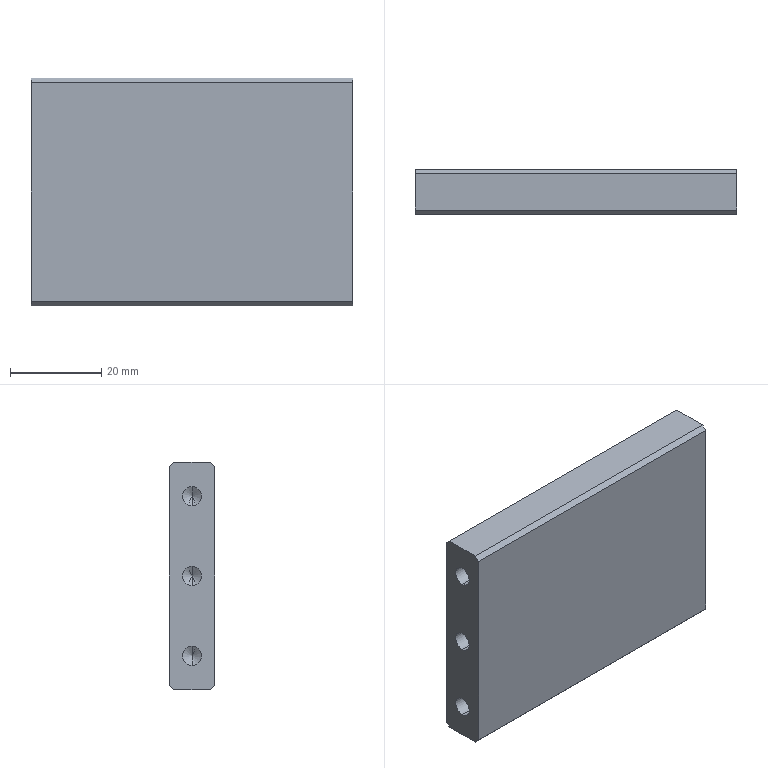Part | STEP file | 10000020443swp000-1 | 1 solid | 34 faces | box 70.5 x 10 x 50 mm | volume 33628 mm3 | cylinder 12 | cone 12 | plane 10 | commonest cylinder face diameters 4.2 x12
STEP:
#1=CARTESIAN_POINT('',(-17.85,5.,15.4));
#2=VERTEX_POINT('',#1);
#3=CARTESIAN_POINT('',(-17.85,5.,19.6));
#4=VERTEX_POINT('',#3);
#5=CARTESIAN_POINT('',(-17.85,5.,17.5));
#6=DIRECTION('',(-1.,0.,0.));
#7=DIRECTION('',(0.,0.,1.));
#8=AXIS2_PLACEMENT_3D('',#5,#6,#7);
#9=CIRCLE('',#8,2.1);
#10=EDGE_CURVE('',#2,#4,#9,.T.);
#11=ORIENTED_EDGE('',*,*,#10,.F.);
#12=CARTESIAN_POINT('',(-35.25,5.,15.4));
#13=VERTEX_POINT('',#12);
#14=CARTESIAN_POINT('',(-35.25,5.,15.4));
#15=DIRECTION('',(-1.,0.,0.));
#16=VECTOR('',#15,1000.);
#17=LINE('',#14,#16);
#18=EDGE_CURVE('',#2,#13,#17,.T.);
#19=ORIENTED_EDGE('',*,*,#18,.T.);
#20=CARTESIAN_POINT('',(-35.25,5.,19.6));
#21=VERTEX_POINT('',#20);
#22=CARTESIAN_POINT('',(-35.25,5.,17.5));
#23=DIRECTION('',(-1.,0.,0.));
#24=DIRECTION('',(0.,0.,1.));
#25=AXIS2_PLACEMENT_3D('',#22,#23,#24);
#26=CIRCLE('',#25,2.1);
#27=EDGE_CURVE('',#13,#21,#26,.T.);
#28=ORIENTED_EDGE('',*,*,#27,.T.);
#29=CARTESIAN_POINT('',(-35.25,5.,19.6));
#30=DIRECTION('',(-1.,0.,0.));
#31=VECTOR('',#30,1000.);
#32=LINE('',#29,#31);
#33=EDGE_CURVE('',#4,#21,#32,.T.);
#34=ORIENTED_EDGE('',*,*,#33,.F.);
#35=EDGE_LOOP('',(#11,#19,#28,#34));
#36=FACE_OUTER_BOUND('',#35,.T.);
#37=CARTESIAN_POINT('',(-35.25,5.,17.5));
#38=DIRECTION('',(-1.,0.,0.));
#39=DIRECTION('',(0.,0.,1.));
#40=AXIS2_PLACEMENT_3D('',#37,#38,#39);
#41=CYLINDRICAL_SURFACE('',#40,2.1);
#42=ADVANCED_FACE('',(#36),#41,.F.);
#43=CARTESIAN_POINT('',(-16.588,5.,17.5));
#44=VERTEX_POINT('',#43);
#45=CARTESIAN_POINT('',(-17.85,5.,19.6));
#46=DIRECTION('',(-0.515,0.,0.8572));
#47=VECTOR('',#46,1000.);
#48=LINE('',#45,#47);
#49=EDGE_CURVE('',#44,#4,#48,.T.);
#50=ORIENTED_EDGE('',*,*,#49,.F.);
#51=CARTESIAN_POINT('',(-17.85,5.,15.4));
#52=DIRECTION('',(-0.515,0.,-0.8572));
#53=VECTOR('',#52,1000.);
#54=LINE('',#51,#53);
#55=EDGE_CURVE('',#44,#2,#54,.T.);
#56=ORIENTED_EDGE('',*,*,#55,.T.);
#57=ORIENTED_EDGE('',*,*,#10,.T.);
#58=EDGE_LOOP('',(#50,#56,#57));
#59=FACE_OUTER_BOUND('',#58,.T.);
#60=CARTESIAN_POINT('',(-17.85,5.,17.5));
#61=DIRECTION('',(-1.,0.,0.));
#62=DIRECTION('',(0.,0.,1.));
#63=AXIS2_PLACEMENT_3D('',#60,#61,#62);
#64=CONICAL_SURFACE('',#63,2.1,1.03);
#65=ADVANCED_FACE('',(#59),#64,.F.);
#66=CARTESIAN_POINT('',(-17.85,5.,-2.1));
#67=VERTEX_POINT('',#66);
#68=CARTESIAN_POINT('',(-17.85,5.,2.1));
#69=VERTEX_POINT('',#68);
#70=CARTESIAN_POINT('',(-17.85,5.,0.));
#71=DIRECTION('',(-1.,0.,0.));
#72=DIRECTION('',(0.,0.,1.));
#73=AXIS2_PLACEMENT_3D('',#70,#71,#72);
#74=CIRCLE('',#73,2.1);
#75=EDGE_CURVE('',#67,#69,#74,.T.);
#76=ORIENTED_EDGE('',*,*,#75,.F.);
#77=CARTESIAN_POINT('',(-35.25,5.,-2.1));
#78=VERTEX_POINT('',#77);
#79=CARTESIAN_POINT('',(-35.25,5.,-2.1));
#80=DIRECTION('',(-1.,0.,0.));
#81=VECTOR('',#80,1000.);
#82=LINE('',#79,#81);
#83=EDGE_CURVE('',#67,#78,#82,.T.);
#84=ORIENTED_EDGE('',*,*,#83,.T.);
#85=CARTESIAN_POINT('',(-35.25,5.,2.1));
#86=VERTEX_POINT('',#85);
#87=CARTESIAN_POINT('',(-35.25,5.,0.));
#88=DIRECTION('',(-1.,0.,0.));
#89=DIRECTION('',(0.,0.,1.));
#90=AXIS2_PLACEMENT_3D('',#87,#88,#89);
#91=CIRCLE('',#90,2.1);
#92=EDGE_CURVE('',#78,#86,#91,.T.);
#93=ORIENTED_EDGE('',*,*,#92,.T.);
#94=CARTESIAN_POINT('',(-35.25,5.,2.1));
#95=DIRECTION('',(-1.,0.,0.));
#96=VECTOR('',#95,1000.);
#97=LINE('',#94,#96);
#98=EDGE_CURVE('',#69,#86,#97,.T.);
#99=ORIENTED_EDGE('',*,*,#98,.F.);
#100=EDGE_LOOP('',(#76,#84,#93,#99));
#101=FACE_OUTER_BOUND('',#100,.T.);
#102=CARTESIAN_POINT('',(-35.25,5.,0.));
#103=DIRECTION('',(-1.,0.,0.));
#104=DIRECTION('',(0.,0.,1.));
#105=AXIS2_PLACEMENT_3D('',#102,#103,#104);
#106=CYLINDRICAL_SURFACE('',#105,2.1);
#107=ADVANCED_FACE('',(#101),#106,.F.);
#108=CARTESIAN_POINT('',(-16.588,5.,0.));
#109=VERTEX_POINT('',#108);
#110=CARTESIAN_POINT('',(-17.85,5.,2.1));
#111=DIRECTION('',(-0.515,0.,0.8572));
#112=VECTOR('',#111,1000.);
#113=LINE('',#110,#112);
#114=EDGE_CURVE('',#109,#69,#113,.T.);
#115=ORIENTED_EDGE('',*,*,#114,.F.);
#116=CARTESIAN_POINT('',(-17.85,5.,-2.1));
#117=DIRECTION('',(-0.515,0.,-0.8572));
#118=VECTOR('',#117,1000.);
#119=LINE('',#116,#118);
#120=EDGE_CURVE('',#109,#67,#119,.T.);
#121=ORIENTED_EDGE('',*,*,#120,.T.);
#122=ORIENTED_EDGE('',*,*,#75,.T.);
#123=EDGE_LOOP('',(#115,#121,#122));
#124=FACE_OUTER_BOUND('',#123,.T.);
#125=CARTESIAN_POINT('',(-17.85,5.,0.));
#126=DIRECTION('',(-1.,0.,0.));
#127=DIRECTION('',(0.,0.,1.));
#128=AXIS2_PLACEMENT_3D('',#125,#126,#127);
#129=CONICAL_SURFACE('',#128,2.1,1.03);
#130=ADVANCED_FACE('',(#124),#129,.F.);
#131=CARTESIAN_POINT('',(-17.85,5.,-19.6));
#132=VERTEX_POINT('',#131);
#133=CARTESIAN_POINT('',(-17.85,5.,-15.4));
#134=VERTEX_POINT('',#133);
#135=CARTESIAN_POINT('',(-17.85,5.,-17.5));
#136=DIRECTION('',(-1.,0.,0.));
#137=DIRECTION('',(0.,0.,1.));
#138=AXIS2_PLACEMENT_3D('',#135,#136,#137);
#139=CIRCLE('',#138,2.1);
#140=EDGE_CURVE('',#132,#134,#139,.T.);
#141=ORIENTED_EDGE('',*,*,#140,.F.);
#142=CARTESIAN_POINT('',(-35.25,5.,-19.6));
#143=VERTEX_POINT('',#142);
#144=CARTESIAN_POINT('',(-35.25,5.,-19.6));
#145=DIRECTION('',(-1.,0.,0.));
#146=VECTOR('',#145,1000.);
#147=LINE('',#144,#146);
#148=EDGE_CURVE('',#132,#143,#147,.T.);
#149=ORIENTED_EDGE('',*,*,#148,.T.);
#150=CARTESIAN_POINT('',(-35.25,5.,-15.4));
#151=VERTEX_POINT('',#150);
#152=CARTESIAN_POINT('',(-35.25,5.,-17.5));
#153=DIRECTION('',(-1.,0.,0.));
#154=DIRECTION('',(0.,0.,1.));
#155=AXIS2_PLACEMENT_3D('',#152,#153,#154);
#156=CIRCLE('',#155,2.1);
#157=EDGE_CURVE('',#143,#151,#156,.T.);
#158=ORIENTED_EDGE('',*,*,#157,.T.);
#159=CARTESIAN_POINT('',(-35.25,5.,-15.4));
#160=DIRECTION('',(-1.,0.,0.));
#161=VECTOR('',#160,1000.);
#162=LINE('',#159,#161);
#163=EDGE_CURVE('',#134,#151,#162,.T.);
#164=ORIENTED_EDGE('',*,*,#163,.F.);
#165=EDGE_LOOP('',(#141,#149,#158,#164));
#166=FACE_OUTER_BOUND('',#165,.T.);
#167=CARTESIAN_POINT('',(-35.25,5.,-17.5));
#168=DIRECTION('',(-1.,0.,0.));
#169=DIRECTION('',(0.,0.,1.));
#170=AXIS2_PLACEMENT_3D('',#167,#168,#169);
#171=CYLINDRICAL_SURFACE('',#170,2.1);
#172=ADVANCED_FACE('',(#166),#171,.F.);
#173=CARTESIAN_POINT('',(-16.588,5.,-17.5));
#174=VERTEX_POINT('',#173);
#175=CARTESIAN_POINT('',(-17.85,5.,-15.4));
#176=DIRECTION('',(-0.515,0.,0.8572));
#177=VECTOR('',#176,1000.);
#178=LINE('',#175,#177);
#179=EDGE_CURVE('',#174,#134,#178,.T.);
#180=ORIENTED_EDGE('',*,*,#179,.F.);
#181=CARTESIAN_POINT('',(-17.85,5.,-19.6));
#182=DIRECTION('',(-0.515,0.,-0.8572));
#183=VECTOR('',#182,1000.);
#184=LINE('',#181,#183);
#185=EDGE_CURVE('',#174,#132,#184,.T.);
#186=ORIENTED_EDGE('',*,*,#185,.T.);
#187=ORIENTED_EDGE('',*,*,#140,.T.);
#188=EDGE_LOOP('',(#180,#186,#187));
#189=FACE_OUTER_BOUND('',#188,.T.);
#190=CARTESIAN_POINT('',(-17.85,5.,-17.5));
#191=DIRECTION('',(-1.,0.,0.));
#192=DIRECTION('',(0.,0.,1.));
#193=AXIS2_PLACEMENT_3D('',#190,#191,#192);
#194=CONICAL_SURFACE('',#193,2.1,1.03);
#195=ADVANCED_FACE('',(#189),#194,.F.);
#196=CARTESIAN_POINT('',(17.85,5.,19.6));
#197=VERTEX_POINT('',#196);
#198=CARTESIAN_POINT('',(17.85,5.,15.4));
#199=VERTEX_POINT('',#198);
#200=CARTESIAN_POINT('',(17.85,5.,17.5));
#201=DIRECTION('',(1.,0.,0.));
#202=DIRECTION('',(0.,0.,-1.));
#203=AXIS2_PLACEMENT_3D('',#200,#201,#202);
#204=CIRCLE('',#203,2.1);
#205=EDGE_CURVE('',#197,#199,#204,.T.);
#206=ORIENTED_EDGE('',*,*,#205,.F.);
#207=CARTESIAN_POINT('',(35.25,5.,19.6));
#208=VERTEX_POINT('',#207);
#209=CARTESIAN_POINT('',(35.25,5.,19.6));
#210=DIRECTION('',(1.,0.,0.));
#211=VECTOR('',#210,1000.);
#212=LINE('',#209,#211);
#213=EDGE_CURVE('',#197,#208,#212,.T.);
#214=ORIENTED_EDGE('',*,*,#213,.T.);
#215=CARTESIAN_POINT('',(35.25,5.,15.4));
#216=VERTEX_POINT('',#215);
#217=CARTESIAN_POINT('',(35.25,5.,17.5));
#218=DIRECTION('',(1.,0.,0.));
#219=DIRECTION('',(0.,0.,-1.));
#220=AXIS2_PLACEMENT_3D('',#217,#218,#219);
#221=CIRCLE('',#220,2.1);
#222=EDGE_CURVE('',#208,#216,#221,.T.);
#223=ORIENTED_EDGE('',*,*,#222,.T.);
#224=CARTESIAN_POINT('',(35.25,5.,15.4));
#225=DIRECTION('',(1.,0.,0.));
#226=VECTOR('',#225,1000.);
#227=LINE('',#224,#226);
#228=EDGE_CURVE('',#199,#216,#227,.T.);
#229=ORIENTED_EDGE('',*,*,#228,.F.);
#230=EDGE_LOOP('',(#206,#214,#223,#229));
#231=FACE_OUTER_BOUND('',#230,.T.);
#232=CARTESIAN_POINT('',(35.25,5.,17.5));
#233=DIRECTION('',(1.,0.,0.));
#234=DIRECTION('',(0.,0.,-1.));
#235=AXIS2_PLACEMENT_3D('',#232,#233,#234);
#236=CYLINDRICAL_SURFACE('',#235,2.1);
#237=ADVANCED_FACE('',(#231),#236,.F.);
#238=CARTESIAN_POINT('',(16.588,5.,17.5));
#239=VERTEX_POINT('',#238);
#240=CARTESIAN_POINT('',(17.85,5.,15.4));
#241=DIRECTION('',(0.515,0.,-0.8572));
#242=VECTOR('',#241,1000.);
#243=LINE('',#240,#242);
#244=EDGE_CURVE('',#239,#199,#243,.T.);
#245=ORIENTED_EDGE('',*,*,#244,.F.);
#246=CARTESIAN_POINT('',(17.85,5.,19.6));
#247=DIRECTION('',(0.515,0.,0.8572));
#248=VECTOR('',#247,1000.);
#249=LINE('',#246,#248);
#250=EDGE_CURVE('',#239,#197,#249,.T.);
#251=ORIENTED_EDGE('',*,*,#250,.T.);
#252=ORIENTED_EDGE('',*,*,#205,.T.);
#253=EDGE_LOOP('',(#245,#251,#252));
#254=FACE_OUTER_BOUND('',#253,.T.);
#255=CARTESIAN_POINT('',(17.85,5.,17.5));
#256=DIRECTION('',(1.,0.,0.));
#257=DIRECTION('',(0.,0.,-1.));
#258=AXIS2_PLACEMENT_3D('',#255,#256,#257);
#259=CONICAL_SURFACE('',#258,2.1,1.03);
#260=ADVANCED_FACE('',(#254),#259,.F.);
#261=CARTESIAN_POINT('',(17.85,5.,2.1));
#262=VERTEX_POINT('',#261);
#263=CARTESIAN_POINT('',(17.85,5.,-2.1));
#264=VERTEX_POINT('',#263);
#265=CARTESIAN_POINT('',(17.85,5.,0.));
#266=DIRECTION('',(1.,0.,0.));
#267=DIRECTION('',(0.,0.,-1.));
#268=AXIS2_PLACEMENT_3D('',#265,#266,#267);
#269=CIRCLE('',#268,2.1);
#270=EDGE_CURVE('',#262,#264,#269,.T.);
#271=ORIENTED_EDGE('',*,*,#270,.F.);
#272=CARTESIAN_POINT('',(35.25,5.,2.1));
#273=VERTEX_POINT('',#272);
#274=CARTESIAN_POINT('',(35.25,5.,2.1));
#275=DIRECTION('',(1.,0.,0.));
#276=VECTOR('',#275,1000.);
#277=LINE('',#274,#276);
#278=EDGE_CURVE('',#262,#273,#277,.T.);
#279=ORIENTED_EDGE('',*,*,#278,.T.);
#280=CARTESIAN_POINT('',(35.25,5.,-2.1));
#281=VERTEX_POINT('',#280);
#282=CARTESIAN_POINT('',(35.25,5.,0.));
#283=DIRECTION('',(1.,0.,0.));
#284=DIRECTION('',(0.,0.,-1.));
#285=AXIS2_PLACEMENT_3D('',#282,#283,#284);
#286=CIRCLE('',#285,2.1);
#287=EDGE_CURVE('',#273,#281,#286,.T.);
#288=ORIENTED_EDGE('',*,*,#287,.T.);
#289=CARTESIAN_POINT('',(35.25,5.,-2.1));
#290=DIRECTION('',(1.,0.,0.));
#291=VECTOR('',#290,1000.);
#292=LINE('',#289,#291);
#293=EDGE_CURVE('',#264,#281,#292,.T.);
#294=ORIENTED_EDGE('',*,*,#293,.F.);
#295=EDGE_LOOP('',(#271,#279,#288,#294));
#296=FACE_OUTER_BOUND('',#295,.T.);
#297=CARTESIAN_POINT('',(35.25,5.,0.));
#298=DIRECTION('',(1.,0.,0.));
#299=DIRECTION('',(0.,0.,-1.));
#300=AXIS2_PLACEMENT_3D('',#297,#298,#299);
#301=CYLINDRICAL_SURFACE('',#300,2.1);
#302=ADVANCED_FACE('',(#296),#301,.F.);
#303=CARTESIAN_POINT('',(16.588,5.,0.));
#304=VERTEX_POINT('',#303);
#305=CARTESIAN_POINT('',(17.85,5.,-2.1));
#306=DIRECTION('',(0.515,0.,-0.8572));
#307=VECTOR('',#306,1000.);
#308=LINE('',#305,#307);
#309=EDGE_CURVE('',#304,#264,#308,.T.);
#310=ORIENTED_EDGE('',*,*,#309,.F.);
#311=CARTESIAN_POINT('',(17.85,5.,2.1));
#312=DIRECTION('',(0.515,0.,0.8572));
#313=VECTOR('',#312,1000.);
#314=LINE('',#311,#313);
#315=EDGE_CURVE('',#304,#262,#314,.T.);
#316=ORIENTED_EDGE('',*,*,#315,.T.);
#317=ORIENTED_EDGE('',*,*,#270,.T.);
#318=EDGE_LOOP('',(#310,#316,#317));
#319=FACE_OUTER_BOUND('',#318,.T.);
#320=CARTESIAN_POINT('',(17.85,5.,0.));
#321=DIRECTION('',(1.,0.,0.));
#322=DIRECTION('',(0.,0.,-1.));
#323=AXIS2_PLACEMENT_3D('',#320,#321,#322);
#324=CONICAL_SURFACE('',#323,2.1,1.03);
#325=ADVANCED_FACE('',(#319),#324,.F.);
#326=CARTESIAN_POINT('',(17.85,5.,-15.4));
#327=VERTEX_POINT('',#326);
#328=CARTESIAN_POINT('',(17.85,5.,-19.6));
#329=VERTEX_POINT('',#328);
#330=CARTESIAN_POINT('',(17.85,5.,-17.5));
#331=DIRECTION('',(1.,0.,0.));
#332=DIRECTION('',(0.,0.,-1.));
#333=AXIS2_PLACEMENT_3D('',#330,#331,#332);
#334=CIRCLE('',#333,2.1);
#335=EDGE_CURVE('',#327,#329,#334,.T.);
#336=ORIENTED_EDGE('',*,*,#335,.F.);
#337=CARTESIAN_POINT('',(35.25,5.,-15.4));
#338=VERTEX_POINT('',#337);
#339=CARTESIAN_POINT('',(35.25,5.,-15.4));
#340=DIRECTION('',(1.,0.,0.));
#341=VECTOR('',#340,1000.);
#342=LINE('',#339,#341);
#343=EDGE_CURVE('',#327,#338,#342,.T.);
#344=ORIENTED_EDGE('',*,*,#343,.T.);
#345=CARTESIAN_POINT('',(35.25,5.,-19.6));
#346=VERTEX_POINT('',#345);
#347=CARTESIAN_POINT('',(35.25,5.,-17.5));
#348=DIRECTION('',(1.,0.,0.));
#349=DIRECTION('',(0.,0.,-1.));
#350=AXIS2_PLACEMENT_3D('',#347,#348,#349);
#351=CIRCLE('',#350,2.1);
#352=EDGE_CURVE('',#338,#346,#351,.T.);
#353=ORIENTED_EDGE('',*,*,#352,.T.);
#354=CARTESIAN_POINT('',(35.25,5.,-19.6));
#355=DIRECTION('',(1.,0.,0.));
#356=VECTOR('',#355,1000.);
#357=LINE('',#354,#356);
#358=EDGE_CURVE('',#329,#346,#357,.T.);
#359=ORIENTED_EDGE('',*,*,#358,.F.);
#360=EDGE_LOOP('',(#336,#344,#353,#359));
#361=FACE_OUTER_BOUND('',#360,.T.);
#362=CARTESIAN_POINT('',(35.25,5.,-17.5));
#363=DIRECTION('',(1.,0.,0.));
#364=DIRECTION('',(0.,0.,-1.));
#365=AXIS2_PLACEMENT_3D('',#362,#363,#364);
#366=CYLINDRICAL_SURFACE('',#365,2.1);
#367=ADVANCED_FACE('',(#361),#366,.F.);
#368=CARTESIAN_POINT('',(16.588,5.,-17.5));
#369=VERTEX_POINT('',#368);
#370=CARTESIAN_POINT('',(17.85,5.,-19.6));
#371=DIRECTION('',(0.515,0.,-0.8572));
#372=VECTOR('',#371,1000.);
#373=LINE('',#370,#372);
#374=EDGE_CURVE('',#369,#329,#373,.T.);
#375=ORIENTED_EDGE('',*,*,#374,.F.);
#376=CARTESIAN_POINT('',(17.85,5.,-15.4));
#377=DIRECTION('',(0.515,0.,0.8572));
#378=VECTOR('',#377,1000.);
#379=LINE('',#376,#378);
#380=EDGE_CURVE('',#369,#327,#379,.T.);
#381=ORIENTED_EDGE('',*,*,#380,.T.);
#382=ORIENTED_EDGE('',*,*,#335,.T.);
#383=EDGE_LOOP('',(#375,#381,#382));
#384=FACE_OUTER_BOUND('',#383,.T.);
#385=CARTESIAN_POINT('',(17.85,5.,-17.5));
#386=DIRECTION('',(1.,0.,0.));
#387=DIRECTION('',(0.,0.,-1.));
#388=AXIS2_PLACEMENT_3D('',#385,#386,#387);
#389=CONICAL_SURFACE('',#388,2.1,1.03);
#390=ADVANCED_FACE('',(#384),#389,.F.);
#391=CARTESIAN_POINT('',(35.25,5.,17.5));
#392=DIRECTION('',(1.,0.,0.));
#393=DIRECTION('',(0.,0.,-1.));
#394=AXIS2_PLACEMENT_3D('',#391,#392,#393);
#395=CIRCLE('',#394,2.1);
#396=EDGE_CURVE('',#216,#208,#395,.T.);
#397=ORIENTED_EDGE('',*,*,#396,.F.);
#398=ORIENTED_EDGE('',*,*,#222,.F.);
#399=EDGE_LOOP('',(#397,#398));
#400=FACE_BOUND('',#399,.T.);
#401=CARTESIAN_POINT('',(35.25,5.,0.));
#402=DIRECTION('',(1.,0.,0.));
#403=DIRECTION('',(0.,0.,-1.));
#404=AXIS2_PLACEMENT_3D('',#401,#402,#403);
#405=CIRCLE('',#404,2.1);
#406=EDGE_CURVE('',#281,#273,#405,.T.);
#407=ORIENTED_EDGE('',*,*,#406,.F.);
#408=ORIENTED_EDGE('',*,*,#287,.F.);
#409=EDGE_LOOP('',(#407,#408));
#410=FACE_BOUND('',#409,.T.);
#411=CARTESIAN_POINT('',(35.25,5.,-17.5));
#412=DIRECTION('',(1.,0.,0.));
#413=DIRECTION('',(0.,0.,-1.));
#414=AXIS2_PLACEMENT_3D('',#411,#412,#413);
#415=CIRCLE('',#414,2.1);
#416=EDGE_CURVE('',#346,#338,#415,.T.);
#417=ORIENTED_EDGE('',*,*,#416,.F.);
#418=ORIENTED_EDGE('',*,*,#352,.F.);
#419=EDGE_LOOP('',(#417,#418));
#420=FACE_BOUND('',#419,.T.);
#421=CARTESIAN_POINT('',(35.25,0.,24.));
#422=VERTEX_POINT('',#421);
#423=CARTESIAN_POINT('',(35.25,0.,-24.));
#424=VERTEX_POINT('',#423);
#425=CARTESIAN_POINT('',(35.25,0.,-25.));
#426=DIRECTION('',(0.,0.,-1.));
#427=VECTOR('',#426,1000.);
#428=LINE('',#425,#427);
#429=EDGE_CURVE('',#422,#424,#428,.T.);
#430=ORIENTED_EDGE('',*,*,#429,.T.);
#431=CARTESIAN_POINT('',(35.25,1.,-25.));
#432=VERTEX_POINT('',#431);
#433=CARTESIAN_POINT('',(35.25,1.,-25.));
#434=DIRECTION('',(0.,0.7071,-0.7071));
#435=VECTOR('',#434,1000.);
#436=LINE('',#433,#435);
#437=EDGE_CURVE('',#424,#432,#436,.T.);
#438=ORIENTED_EDGE('',*,*,#437,.T.);
#439=CARTESIAN_POINT('',(35.25,9.,-25.));
#440=VERTEX_POINT('',#439);
#441=CARTESIAN_POINT('',(35.25,10.,-25.));
#442=DIRECTION('',(0.,-1.,0.));
#443=VECTOR('',#442,1000.);
#444=LINE('',#441,#443);
#445=EDGE_CURVE('',#440,#432,#444,.T.);
#446=ORIENTED_EDGE('',*,*,#445,.F.);
#447=CARTESIAN_POINT('',(35.25,10.,-24.));
#448=VERTEX_POINT('',#447);
#449=CARTESIAN_POINT('',(35.25,10.,-24.));
#450=DIRECTION('',(0.,0.7071,0.7071));
#451=VECTOR('',#450,1000.);
#452=LINE('',#449,#451);
#453=EDGE_CURVE('',#440,#448,#452,.T.);
#454=ORIENTED_EDGE('',*,*,#453,.T.);
#455=CARTESIAN_POINT('',(35.25,10.,24.));
#456=VERTEX_POINT('',#455);
#457=CARTESIAN_POINT('',(35.25,10.,-25.));
#458=DIRECTION('',(0.,0.,-1.));
#459=VECTOR('',#458,1000.);
#460=LINE('',#457,#459);
#461=EDGE_CURVE('',#456,#448,#460,.T.);
#462=ORIENTED_EDGE('',*,*,#461,.F.);
#463=CARTESIAN_POINT('',(35.25,9.,25.));
#464=VERTEX_POINT('',#463);
#465=CARTESIAN_POINT('',(35.25,10.,24.));
#466=DIRECTION('',(0.,-0.7071,0.7071));
#467=VECTOR('',#466,1000.);
#468=LINE('',#465,#467);
#469=EDGE_CURVE('',#456,#464,#468,.T.);
#470=ORIENTED_EDGE('',*,*,#469,.T.);
#471=CARTESIAN_POINT('',(35.25,1.,25.));
#472=VERTEX_POINT('',#471);
#473=CARTESIAN_POINT('',(35.25,10.,25.));
#474=DIRECTION('',(0.,-1.,0.));
#475=VECTOR('',#474,1000.);
#476=LINE('',#473,#475);
#477=EDGE_CURVE('',#464,#472,#476,.T.);
#478=ORIENTED_EDGE('',*,*,#477,.T.);
#479=CARTESIAN_POINT('',(35.25,1.,25.));
#480=DIRECTION('',(0.,-0.7071,-0.7071));
#481=VECTOR('',#480,1000.);
#482=LINE('',#479,#481);
#483=EDGE_CURVE('',#472,#422,#482,.T.);
#484=ORIENTED_EDGE('',*,*,#483,.T.);
#485=EDGE_LOOP('',(#430,#438,#446,#454,#462,#470,#478,#484));
#486=FACE_OUTER_BOUND('',#485,.T.);
#487=CARTESIAN_POINT('',(35.25,10.,-25.));
#488=DIRECTION('',(-1.,0.,0.));
#489=DIRECTION('',(0.,0.,1.));
#490=AXIS2_PLACEMENT_3D('',#487,#488,#489);
#491=PLANE('',#490);
#492=ADVANCED_FACE('',(#400,#410,#420,#486),#491,.F.);
#493=ORIENTED_EDGE('',*,*,#445,.T.);
#494=CARTESIAN_POINT('',(-35.25,1.,-25.));
#495=VERTEX_POINT('',#494);
#496=CARTESIAN_POINT('',(-35.25,1.,-25.));
#497=DIRECTION('',(-1.,0.,0.));
#498=VECTOR('',#497,1000.);
#499=LINE('',#496,#498);
#500=EDGE_CURVE('',#432,#495,#499,.T.);
#501=ORIENTED_EDGE('',*,*,#500,.T.);
#502=CARTESIAN_POINT('',(-35.25,9.,-25.));
#503=VERTEX_POINT('',#502);
#504=CARTESIAN_POINT('',(-35.25,10.,-25.));
#505=DIRECTION('',(0.,-1.,0.));
#506=VECTOR('',#505,1000.);
#507=LINE('',#504,#506);
#508=EDGE_CURVE('',#503,#495,#507,.T.);
#509=ORIENTED_EDGE('',*,*,#508,.F.);
#510=CARTESIAN_POINT('',(35.25,9.,-25.));
#511=DIRECTION('',(1.,0.,0.));
#512=VECTOR('',#511,1000.);
#513=LINE('',#510,#512);
#514=EDGE_CURVE('',#503,#440,#513,.T.);
#515=ORIENTED_EDGE('',*,*,#514,.T.);
#516=EDGE_LOOP('',(#493,#501,#509,#515));
#517=FACE_OUTER_BOUND('',#516,.T.);
#518=CARTESIAN_POINT('',(-35.25,10.,-25.));
#519=DIRECTION('',(0.,0.,1.));
#520=DIRECTION('',(1.,0.,0.));
#521=AXIS2_PLACEMENT_3D('',#518,#519,#520);
#522=PLANE('',#521);
#523=ADVANCED_FACE('',(#517),#522,.F.);
#524=CARTESIAN_POINT('',(-35.25,5.,17.5));
#525=DIRECTION('',(-1.,0.,0.));
#526=DIRECTION('',(0.,0.,1.));
#527=AXIS2_PLACEMENT_3D('',#524,#525,#526);
#528=CIRCLE('',#527,2.1);
#529=EDGE_CURVE('',#21,#13,#528,.T.);
#530=ORIENTED_EDGE('',*,*,#529,.F.);
#531=ORIENTED_EDGE('',*,*,#27,.F.);
#532=EDGE_LOOP('',(#530,#531));
#533=FACE_BOUND('',#532,.T.);
#534=CARTESIAN_POINT('',(-35.25,5.,0.));
#535=DIRECTION('',(-1.,0.,0.));
#536=DIRECTION('',(0.,0.,1.));
#537=AXIS2_PLACEMENT_3D('',#534,#535,#536);
#538=CIRCLE('',#537,2.1);
#539=EDGE_CURVE('',#86,#78,#538,.T.);
#540=ORIENTED_EDGE('',*,*,#539,.F.);
#541=ORIENTED_EDGE('',*,*,#92,.F.);
#542=EDGE_LOOP('',(#540,#541));
#543=FACE_BOUND('',#542,.T.);
#544=CARTESIAN_POINT('',(-35.25,5.,-17.5));
#545=DIRECTION('',(-1.,0.,0.));
#546=DIRECTION('',(0.,0.,1.));
#547=AXIS2_PLACEMENT_3D('',#544,#545,#546);
#548=CIRCLE('',#547,2.1);
#549=EDGE_CURVE('',#151,#143,#548,.T.);
#550=ORIENTED_EDGE('',*,*,#549,.F.);
#551=ORIENTED_EDGE('',*,*,#157,.F.);
#552=EDGE_LOOP('',(#550,#551));
#553=FACE_BOUND('',#552,.T.);
#554=ORIENTED_EDGE('',*,*,#508,.T.);
#555=CARTESIAN_POINT('',(-35.25,0.,-24.));
#556=VERTEX_POINT('',#555);
#557=CARTESIAN_POINT('',(-35.25,1.,-25.));
#558=DIRECTION('',(0.,-0.7071,0.7071));
#559=VECTOR('',#558,1000.);
#560=LINE('',#557,#559);
#561=EDGE_CURVE('',#495,#556,#560,.T.);
#562=ORIENTED_EDGE('',*,*,#561,.T.);
#563=CARTESIAN_POINT('',(-35.25,0.,24.));
#564=VERTEX_POINT('',#563);
#565=CARTESIAN_POINT('',(-35.25,0.,-25.));
#566=DIRECTION('',(0.,0.,1.));
#567=VECTOR('',#566,1000.);
#568=LINE('',#565,#567);
#569=EDGE_CURVE('',#556,#564,#568,.T.);
#570=ORIENTED_EDGE('',*,*,#569,.T.);
#571=CARTESIAN_POINT('',(-35.25,1.,25.));
#572=VERTEX_POINT('',#571);
#573=CARTESIAN_POINT('',(-35.25,1.,25.));
#574=DIRECTION('',(0.,0.7071,0.7071));
#575=VECTOR('',#574,1000.);
#576=LINE('',#573,#575);
#577=EDGE_CURVE('',#564,#572,#576,.T.);
#578=ORIENTED_EDGE('',*,*,#577,.T.);
#579=CARTESIAN_POINT('',(-35.25,9.,25.));
#580=VERTEX_POINT('',#579);
#581=CARTESIAN_POINT('',(-35.25,10.,25.));
#582=DIRECTION('',(0.,-1.,0.));
#583=VECTOR('',#582,1000.);
#584=LINE('',#581,#583);
#585=EDGE_CURVE('',#580,#572,#584,.T.);
#586=ORIENTED_EDGE('',*,*,#585,.F.);
#587=CARTESIAN_POINT('',(-35.25,10.,24.));
#588=VERTEX_POINT('',#587);
#589=CARTESIAN_POINT('',(-35.25,10.,24.));
#590=DIRECTION('',(0.,0.7071,-0.7071));
#591=VECTOR('',#590,1000.);
#592=LINE('',#589,#591);
#593=EDGE_CURVE('',#580,#588,#592,.T.);
#594=ORIENTED_EDGE('',*,*,#593,.T.);
#595=CARTESIAN_POINT('',(-35.25,10.,-24.));
#596=VERTEX_POINT('',#595);
#597=CARTESIAN_POINT('',(-35.25,10.,-25.));
#598=DIRECTION('',(0.,0.,1.));
#599=VECTOR('',#598,1000.);
#600=LINE('',#597,#599);
#601=EDGE_CURVE('',#596,#588,#600,.T.);
#602=ORIENTED_EDGE('',*,*,#601,.F.);
#603=CARTESIAN_POINT('',(-35.25,10.,-24.));
#604=DIRECTION('',(0.,-0.7071,-0.7071));
#605=VECTOR('',#604,1000.);
#606=LINE('',#603,#605);
#607=EDGE_CURVE('',#596,#503,#606,.T.);
#608=ORIENTED_EDGE('',*,*,#607,.T.);
#609=EDGE_LOOP('',(#554,#562,#570,#578,#586,#594,#602,#608));
#610=FACE_OUTER_BOUND('',#609,.T.);
#611=CARTESIAN_POINT('',(-35.25,10.,-25.));
#612=DIRECTION('',(1.,0.,0.));
#613=DIRECTION('',(0.,0.,-1.));
#614=AXIS2_PLACEMENT_3D('',#611,#612,#613);
#615=PLANE('',#614);
#616=ADVANCED_FACE('',(#533,#543,#553,#610),#615,.F.);
#617=ORIENTED_EDGE('',*,*,#585,.T.);
#618=CARTESIAN_POINT('',(-35.25,1.,25.));
#619=DIRECTION('',(1.,0.,0.));
#620=VECTOR('',#619,1000.);
#621=LINE('',#618,#620);
#622=EDGE_CURVE('',#572,#472,#621,.T.);
#623=ORIENTED_EDGE('',*,*,#622,.T.);
#624=ORIENTED_EDGE('',*,*,#477,.F.);
#625=CARTESIAN_POINT('',(-35.25,9.,25.));
#626=DIRECTION('',(-1.,0.,0.));
#627=VECTOR('',#626,1000.);
#628=LINE('',#625,#627);
#629=EDGE_CURVE('',#464,#580,#628,.T.);
#630=ORIENTED_EDGE('',*,*,#629,.T.);
#631=EDGE_LOOP('',(#617,#623,#624,#630));
#632=FACE_OUTER_BOUND('',#631,.T.);
#633=CARTESIAN_POINT('',(-35.25,10.,25.));
#634=DIRECTION('',(0.,0.,-1.));
#635=DIRECTION('',(-1.,0.,0.));
#636=AXIS2_PLACEMENT_3D('',#633,#634,#635);
#637=PLANE('',#636);
#638=ADVANCED_FACE('',(#632),#637,.F.);
#639=ORIENTED_EDGE('',*,*,#461,.T.);
#640=CARTESIAN_POINT('',(-35.25,10.,-24.));
#641=DIRECTION('',(-1.,0.,0.));
#642=VECTOR('',#641,1000.);
#643=LINE('',#640,#642);
#644=EDGE_CURVE('',#448,#596,#643,.T.);
#645=ORIENTED_EDGE('',*,*,#644,.T.);
#646=ORIENTED_EDGE('',*,*,#601,.T.);
#647=CARTESIAN_POINT('',(35.25,10.,24.));
#648=DIRECTION('',(1.,0.,0.));
#649=VECTOR('',#648,1000.);
#650=LINE('',#647,#649);
#651=EDGE_CURVE('',#588,#456,#650,.T.);
#652=ORIENTED_EDGE('',*,*,#651,.T.);
#653=EDGE_LOOP('',(#639,#645,#646,#652));
#654=FACE_OUTER_BOUND('',#653,.T.);
#655=CARTESIAN_POINT('',(0.,10.,0.));
#656=DIRECTION('',(0.,1.,0.));
#657=DIRECTION('',(0.,0.,1.));
#658=AXIS2_PLACEMENT_3D('',#655,#656,#657);
#659=PLANE('',#658);
#660=ADVANCED_FACE('',(#654),#659,.T.);
#661=ORIENTED_EDGE('',*,*,#569,.F.);
#662=CARTESIAN_POINT('',(0.,0.,-24.));
#663=DIRECTION('',(1.,0.,0.));
#664=VECTOR('',#663,1000.);
#665=LINE('',#662,#664);
#666=EDGE_CURVE('',#556,#424,#665,.T.);
#667=ORIENTED_EDGE('',*,*,#666,.T.);
#668=ORIENTED_EDGE('',*,*,#429,.F.);
#669=CARTESIAN_POINT('',(0.,0.,24.));
#670=DIRECTION('',(-1.,0.,0.));
#671=VECTOR('',#670,1000.);
#672=LINE('',#669,#671);
#673=EDGE_CURVE('',#422,#564,#672,.T.);
#674=ORIENTED_EDGE('',*,*,#673,.T.);
#675=EDGE_LOOP('',(#661,#667,#668,#674));
#676=FACE_OUTER_BOUND('',#675,.T.);
#677=CARTESIAN_POINT('',(0.,0.,0.));
#678=DIRECTION('',(0.,1.,0.));
#679=DIRECTION('',(0.,0.,1.));
#680=AXIS2_PLACEMENT_3D('',#677,#678,#679);
#681=PLANE('',#680);
#682=ADVANCED_FACE('',(#676),#681,.F.);
#683=ORIENTED_EDGE('',*,*,#380,.F.);
#684=ORIENTED_EDGE('',*,*,#374,.T.);
#685=CARTESIAN_POINT('',(17.85,5.,-17.5));
#686=DIRECTION('',(1.,0.,0.));
#687=DIRECTION('',(0.,0.,-1.));
#688=AXIS2_PLACEMENT_3D('',#685,#686,#687);
#689=CIRCLE('',#688,2.1);
#690=EDGE_CURVE('',#329,#327,#689,.T.);
#691=ORIENTED_EDGE('',*,*,#690,.T.);
#692=EDGE_LOOP('',(#683,#684,#691));
#693=FACE_OUTER_BOUND('',#692,.T.);
#694=CARTESIAN_POINT('',(17.85,5.,-17.5));
#695=DIRECTION('',(1.,0.,0.));
#696=DIRECTION('',(0.,0.,-1.));
#697=AXIS2_PLACEMENT_3D('',#694,#695,#696);
#698=CONICAL_SURFACE('',#697,2.1,1.03);
#699=ADVANCED_FACE('',(#693),#698,.F.);
#700=ORIENTED_EDGE('',*,*,#343,.F.);
#701=ORIENTED_EDGE('',*,*,#690,.F.);
#702=ORIENTED_EDGE('',*,*,#358,.T.);
#703=ORIENTED_EDGE('',*,*,#416,.T.);
#704=EDGE_LOOP('',(#700,#701,#702,#703));
#705=FACE_OUTER_BOUND('',#704,.T.);
#706=CARTESIAN_POINT('',(35.25,5.,-17.5));
#707=DIRECTION('',(1.,0.,0.));
#708=DIRECTION('',(0.,0.,-1.));
#709=AXIS2_PLACEMENT_3D('',#706,#707,#708);
#710=CYLINDRICAL_SURFACE('',#709,2.1);
#711=ADVANCED_FACE('',(#705),#710,.F.);
#712=ORIENTED_EDGE('',*,*,#315,.F.);
#713=ORIENTED_EDGE('',*,*,#309,.T.);
#714=CARTESIAN_POINT('',(17.85,5.,0.));
#715=DIRECTION('',(1.,0.,0.));
#716=DIRECTION('',(0.,0.,-1.));
#717=AXIS2_PLACEMENT_3D('',#714,#715,#716);
#718=CIRCLE('',#717,2.1);
#719=EDGE_CURVE('',#264,#262,#718,.T.);
#720=ORIENTED_EDGE('',*,*,#719,.T.);
#721=EDGE_LOOP('',(#712,#713,#720));
#722=FACE_OUTER_BOUND('',#721,.T.);
#723=CARTESIAN_POINT('',(17.85,5.,0.));
#724=DIRECTION('',(1.,0.,0.));
#725=DIRECTION('',(0.,0.,-1.));
#726=AXIS2_PLACEMENT_3D('',#723,#724,#725);
#727=CONICAL_SURFACE('',#726,2.1,1.03);
#728=ADVANCED_FACE('',(#722),#727,.F.);
#729=ORIENTED_EDGE('',*,*,#278,.F.);
#730=ORIENTED_EDGE('',*,*,#719,.F.);
#731=ORIENTED_EDGE('',*,*,#293,.T.);
#732=ORIENTED_EDGE('',*,*,#406,.T.);
#733=EDGE_LOOP('',(#729,#730,#731,#732));
#734=FACE_OUTER_BOUND('',#733,.T.);
#735=CARTESIAN_POINT('',(35.25,5.,0.));
#736=DIRECTION('',(1.,0.,0.));
#737=DIRECTION('',(0.,0.,-1.));
#738=AXIS2_PLACEMENT_3D('',#735,#736,#737);
#739=CYLINDRICAL_SURFACE('',#738,2.1);
#740=ADVANCED_FACE('',(#734),#739,.F.);
#741=ORIENTED_EDGE('',*,*,#250,.F.);
#742=ORIENTED_EDGE('',*,*,#244,.T.);
#743=CARTESIAN_POINT('',(17.85,5.,17.5));
#744=DIRECTION('',(1.,0.,0.));
#745=DIRECTION('',(0.,0.,-1.));
#746=AXIS2_PLACEMENT_3D('',#743,#744,#745);
#747=CIRCLE('',#746,2.1);
#748=EDGE_CURVE('',#199,#197,#747,.T.);
#749=ORIENTED_EDGE('',*,*,#748,.T.);
#750=EDGE_LOOP('',(#741,#742,#749));
#751=FACE_OUTER_BOUND('',#750,.T.);
#752=CARTESIAN_POINT('',(17.85,5.,17.5));
#753=DIRECTION('',(1.,0.,0.));
#754=DIRECTION('',(0.,0.,-1.));
#755=AXIS2_PLACEMENT_3D('',#752,#753,#754);
#756=CONICAL_SURFACE('',#755,2.1,1.03);
#757=ADVANCED_FACE('',(#751),#756,.F.);
#758=ORIENTED_EDGE('',*,*,#213,.F.);
#759=ORIENTED_EDGE('',*,*,#748,.F.);
#760=ORIENTED_EDGE('',*,*,#228,.T.);
#761=ORIENTED_EDGE('',*,*,#396,.T.);
#762=EDGE_LOOP('',(#758,#759,#760,#761));
#763=FACE_OUTER_BOUND('',#762,.T.);
#764=CARTESIAN_POINT('',(35.25,5.,17.5));
#765=DIRECTION('',(1.,0.,0.));
#766=DIRECTION('',(0.,0.,-1.));
#767=AXIS2_PLACEMENT_3D('',#764,#765,#766);
#768=CYLINDRICAL_SURFACE('',#767,2.1);
#769=ADVANCED_FACE('',(#763),#768,.F.);
#770=ORIENTED_EDGE('',*,*,#185,.F.);
#771=ORIENTED_EDGE('',*,*,#179,.T.);
#772=CARTESIAN_POINT('',(-17.85,5.,-17.5));
#773=DIRECTION('',(-1.,0.,0.));
#774=DIRECTION('',(0.,0.,1.));
#775=AXIS2_PLACEMENT_3D('',#772,#773,#774);
#776=CIRCLE('',#775,2.1);
#777=EDGE_CURVE('',#134,#132,#776,.T.);
#778=ORIENTED_EDGE('',*,*,#777,.T.);
#779=EDGE_LOOP('',(#770,#771,#778));
#780=FACE_OUTER_BOUND('',#779,.T.);
#781=CARTESIAN_POINT('',(-17.85,5.,-17.5));
#782=DIRECTION('',(-1.,0.,0.));
#783=DIRECTION('',(0.,0.,1.));
#784=AXIS2_PLACEMENT_3D('',#781,#782,#783);
#785=CONICAL_SURFACE('',#784,2.1,1.03);
#786=ADVANCED_FACE('',(#780),#785,.F.);
#787=ORIENTED_EDGE('',*,*,#148,.F.);
#788=ORIENTED_EDGE('',*,*,#777,.F.);
#789=ORIENTED_EDGE('',*,*,#163,.T.);
#790=ORIENTED_EDGE('',*,*,#549,.T.);
#791=EDGE_LOOP('',(#787,#788,#789,#790));
#792=FACE_OUTER_BOUND('',#791,.T.);
#793=CARTESIAN_POINT('',(-35.25,5.,-17.5));
#794=DIRECTION('',(-1.,0.,0.));
#795=DIRECTION('',(0.,0.,1.));
#796=AXIS2_PLACEMENT_3D('',#793,#794,#795);
#797=CYLINDRICAL_SURFACE('',#796,2.1);
#798=ADVANCED_FACE('',(#792),#797,.F.);
#799=ORIENTED_EDGE('',*,*,#120,.F.);
#800=ORIENTED_EDGE('',*,*,#114,.T.);
#801=CARTESIAN_POINT('',(-17.85,5.,0.));
#802=DIRECTION('',(-1.,0.,0.));
#803=DIRECTION('',(0.,0.,1.));
#804=AXIS2_PLACEMENT_3D('',#801,#802,#803);
#805=CIRCLE('',#804,2.1);
#806=EDGE_CURVE('',#69,#67,#805,.T.);
#807=ORIENTED_EDGE('',*,*,#806,.T.);
#808=EDGE_LOOP('',(#799,#800,#807));
#809=FACE_OUTER_BOUND('',#808,.T.);
#810=CARTESIAN_POINT('',(-17.85,5.,0.));
#811=DIRECTION('',(-1.,0.,0.));
#812=DIRECTION('',(0.,0.,1.));
#813=AXIS2_PLACEMENT_3D('',#810,#811,#812);
#814=CONICAL_SURFACE('',#813,2.1,1.03);
#815=ADVANCED_FACE('',(#809),#814,.F.);
#816=ORIENTED_EDGE('',*,*,#83,.F.);
#817=ORIENTED_EDGE('',*,*,#806,.F.);
#818=ORIENTED_EDGE('',*,*,#98,.T.);
#819=ORIENTED_EDGE('',*,*,#539,.T.);
#820=EDGE_LOOP('',(#816,#817,#818,#819));
#821=FACE_OUTER_BOUND('',#820,.T.);
#822=CARTESIAN_POINT('',(-35.25,5.,0.));
#823=DIRECTION('',(-1.,0.,0.));
#824=DIRECTION('',(0.,0.,1.));
#825=AXIS2_PLACEMENT_3D('',#822,#823,#824);
#826=CYLINDRICAL_SURFACE('',#825,2.1);
#827=ADVANCED_FACE('',(#821),#826,.F.);
#828=ORIENTED_EDGE('',*,*,#55,.F.);
#829=ORIENTED_EDGE('',*,*,#49,.T.);
#830=CARTESIAN_POINT('',(-17.85,5.,17.5));
#831=DIRECTION('',(-1.,0.,0.));
#832=DIRECTION('',(0.,0.,1.));
#833=AXIS2_PLACEMENT_3D('',#830,#831,#832);
#834=CIRCLE('',#833,2.1);
#835=EDGE_CURVE('',#4,#2,#834,.T.);
#836=ORIENTED_EDGE('',*,*,#835,.T.);
#837=EDGE_LOOP('',(#828,#829,#836));
#838=FACE_OUTER_BOUND('',#837,.T.);
#839=CARTESIAN_POINT('',(-17.85,5.,17.5));
#840=DIRECTION('',(-1.,0.,0.));
#841=DIRECTION('',(0.,0.,1.));
#842=AXIS2_PLACEMENT_3D('',#839,#840,#841);
#843=CONICAL_SURFACE('',#842,2.1,1.03);
#844=ADVANCED_FACE('',(#838),#843,.F.);
#845=ORIENTED_EDGE('',*,*,#18,.F.);
#846=ORIENTED_EDGE('',*,*,#835,.F.);
#847=ORIENTED_EDGE('',*,*,#33,.T.);
#848=ORIENTED_EDGE('',*,*,#529,.T.);
#849=EDGE_LOOP('',(#845,#846,#847,#848));
#850=FACE_OUTER_BOUND('',#849,.T.);
#851=CARTESIAN_POINT('',(-35.25,5.,17.5));
#852=DIRECTION('',(-1.,0.,0.));
#853=DIRECTION('',(0.,0.,1.));
#854=AXIS2_PLACEMENT_3D('',#851,#852,#853);
#855=CYLINDRICAL_SURFACE('',#854,2.1);
#856=ADVANCED_FACE('',(#850),#855,.F.);
#857=ORIENTED_EDGE('',*,*,#437,.F.);
#858=ORIENTED_EDGE('',*,*,#666,.F.);
#859=ORIENTED_EDGE('',*,*,#561,.F.);
#860=ORIENTED_EDGE('',*,*,#500,.F.);
#861=EDGE_LOOP('',(#857,#858,#859,#860));
#862=FACE_OUTER_BOUND('',#861,.T.);
#863=CARTESIAN_POINT('',(-35.25,1.,-25.));
#864=DIRECTION('',(0.,0.7071,0.7071));
#865=DIRECTION('',(-1.,0.,0.));
#866=AXIS2_PLACEMENT_3D('',#863,#864,#865);
#867=PLANE('',#866);
#868=ADVANCED_FACE('',(#862),#867,.F.);
#869=ORIENTED_EDGE('',*,*,#453,.F.);
#870=ORIENTED_EDGE('',*,*,#514,.F.);
#871=ORIENTED_EDGE('',*,*,#607,.F.);
#872=ORIENTED_EDGE('',*,*,#644,.F.);
#873=EDGE_LOOP('',(#869,#870,#871,#872));
#874=FACE_OUTER_BOUND('',#873,.T.);
#875=CARTESIAN_POINT('',(0.,10.,-24.));
#876=DIRECTION('',(0.,0.7071,-0.7071));
#877=DIRECTION('',(1.,0.,0.));
#878=AXIS2_PLACEMENT_3D('',#875,#876,#877);
#879=PLANE('',#878);
#880=ADVANCED_FACE('',(#874),#879,.T.);
#881=ORIENTED_EDGE('',*,*,#577,.F.);
#882=ORIENTED_EDGE('',*,*,#673,.F.);
#883=ORIENTED_EDGE('',*,*,#483,.F.);
#884=ORIENTED_EDGE('',*,*,#622,.F.);
#885=EDGE_LOOP('',(#881,#882,#883,#884));
#886=FACE_OUTER_BOUND('',#885,.T.);
#887=CARTESIAN_POINT('',(-35.25,1.,25.));
#888=DIRECTION('',(0.,0.7071,-0.7071));
#889=DIRECTION('',(1.,0.,0.));
#890=AXIS2_PLACEMENT_3D('',#887,#888,#889);
#891=PLANE('',#890);
#892=ADVANCED_FACE('',(#886),#891,.F.);
#893=ORIENTED_EDGE('',*,*,#593,.F.);
#894=ORIENTED_EDGE('',*,*,#629,.F.);
#895=ORIENTED_EDGE('',*,*,#469,.F.);
#896=ORIENTED_EDGE('',*,*,#651,.F.);
#897=EDGE_LOOP('',(#893,#894,#895,#896));
#898=FACE_OUTER_BOUND('',#897,.T.);
#899=CARTESIAN_POINT('',(0.,10.,24.));
#900=DIRECTION('',(0.,0.7071,0.7071));
#901=DIRECTION('',(-1.,0.,0.));
#902=AXIS2_PLACEMENT_3D('',#899,#900,#901);
#903=PLANE('',#902);
#904=ADVANCED_FACE('',(#898),#903,.T.);
#905=CLOSED_SHELL('',(#42,#65,#107,#130,#172,#195,#237,#260,#302,#325,#367,#390,#492,#523,#616,#638,#660,#682,#699,#711,#728,#740,#757,#769,#786,#798,#815,#827,#844,#856,#868,#880,#892,#904));
#906=MANIFOLD_SOLID_BREP('',#905);
#907=CARTESIAN_POINT('',(0.,0.,0.));
#908=DIRECTION('',(0.,0.,1.));
#909=DIRECTION('',(1.,0.,0.));
#910=AXIS2_PLACEMENT_3D('',#907,#908,#909);
#911=(LENGTH_UNIT()NAMED_UNIT(*)SI_UNIT(.MILLI.,.METRE.));
#912=UNCERTAINTY_MEASURE_WITH_UNIT(LENGTH_MEASURE(0.00001),#911,'','');
#913=(NAMED_UNIT(*)PLANE_ANGLE_UNIT()SI_UNIT($,.RADIAN.));
#914=(NAMED_UNIT(*)SI_UNIT($,.STERADIAN.)SOLID_ANGLE_UNIT());
#915=(GEOMETRIC_REPRESENTATION_CONTEXT(3)GLOBAL_UNCERTAINTY_ASSIGNED_CONTEXT((#912))GLOBAL_UNIT_ASSIGNED_CONTEXT((#911,#913,#914))REPRESENTATION_CONTEXT('',''));
#916=ADVANCED_BREP_SHAPE_REPRESENTATION('',(#906,#910),#915);